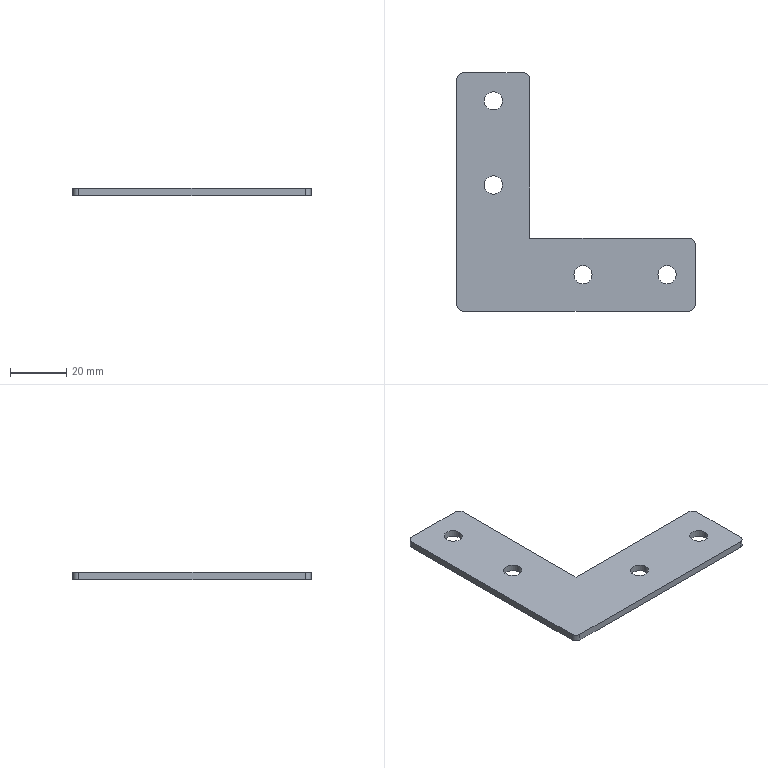Part | STEP file | 3030 L-profile sheet metal | 1 solid | 21 faces | box 85 x 85 x 2.5 mm | volume 9017 mm3 | cylinder 13 | plane 8 | commonest cylinder face diameters 6.5 x8 4 x5